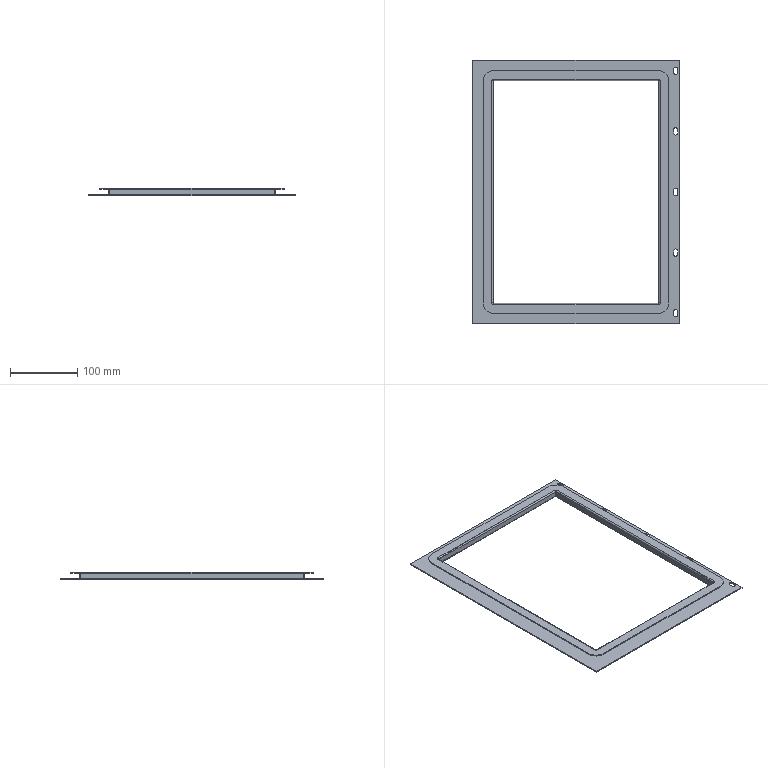Part | SolidWorks | features BaseBody 1 | 1 solid | 88 faces | box 306 x 391 x 11.5 mm | volume 96676 mm3 | plane 42 | cylinder 30 | torus 8 | spline 8 | commonest cylinder face diameters 6 x10 1 x8 4 x8 31.414 x4